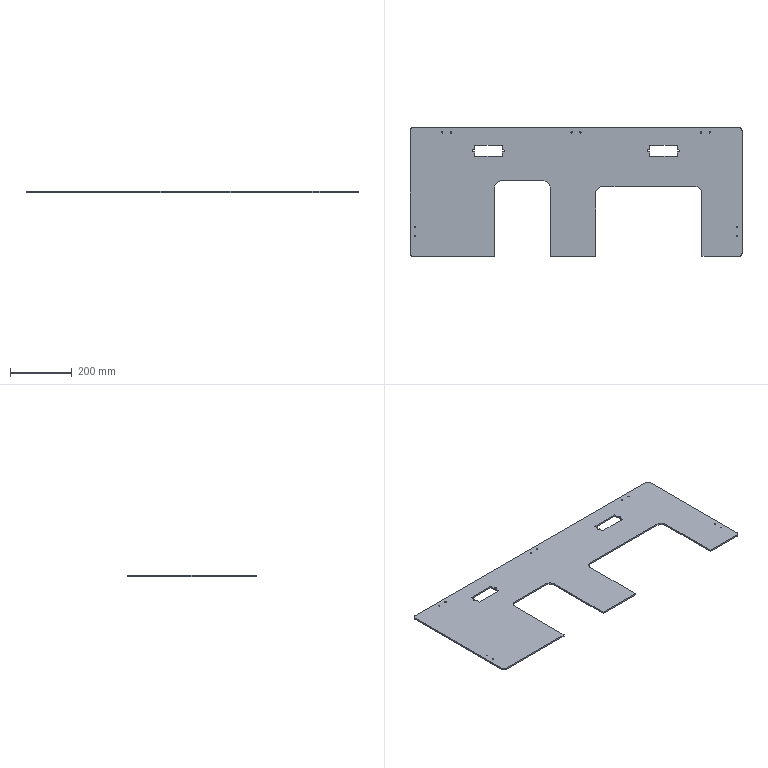Part | STEP file | 09-29 front panel A | 1 solid | 68 faces | box 1078 x 418 x 5 mm | volume 1609737 mm3 | cylinder 34 | plane 34 | commonest cylinder face diameters 4.2 x20 8 x6 20 x4 40 x4